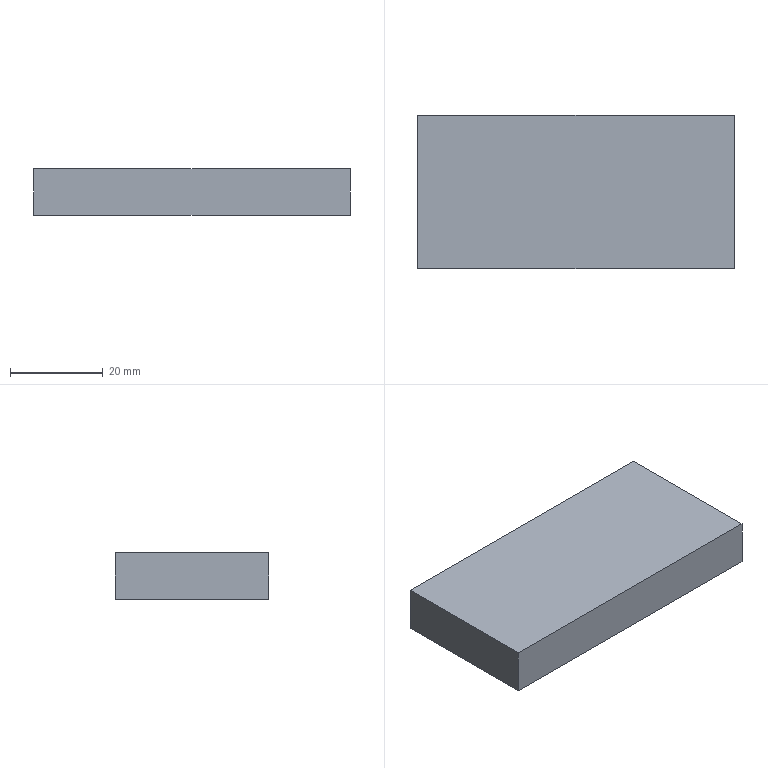Part | STEP file | Display 1 | 1 solid | 6 faces | box 68 x 33 x 10 mm | volume 22440 mm3 | plane 6
STEP:
#1=CARTESIAN_POINT('',(0.,0.,0.));
#2=DIRECTION('',(0.,0.,1.));
#3=DIRECTION('',(1.,0.,0.));
#4=AXIS2_PLACEMENT_3D('',#1,#2,#3);
#5=CARTESIAN_POINT('',(34.,-16.5,10.));
#6=VERTEX_POINT('',#5);
#7=CARTESIAN_POINT('',(34.,16.5,10.));
#8=VERTEX_POINT('',#7);
#9=CARTESIAN_POINT('',(34.,-16.5,10.));
#10=DIRECTION('',(0.,1.,0.));
#11=VECTOR('',#10,1.);
#12=LINE('',#9,#11);
#13=CARTESIAN_POINT('',(-34.,-16.5,10.));
#14=DIRECTION('',(0.,0.,1.));
#15=DIRECTION('',(1.,0.,0.));
#16=AXIS2_PLACEMENT_3D('',#13,#14,#15);
#17=PLANE('',#16);
#18=CARTESIAN_POINT('',(68.,0.));
#19=DIRECTION('',(0.,1.));
#20=VECTOR('',#19,1.);
#21=LINE('',#18,#20);
#22=(GEOMETRIC_REPRESENTATION_CONTEXT(2)PARAMETRIC_REPRESENTATION_CONTEXT()REPRESENTATION_CONTEXT('',''));
#23=DEFINITIONAL_REPRESENTATION('',(#21),#22);
#24=PCURVE('',#17,#23);
#25=CARTESIAN_POINT('',(34.,16.5,10.));
#26=DIRECTION('',(-1.,0.,0.));
#27=DIRECTION('',(0.,-1.,0.));
#28=AXIS2_PLACEMENT_3D('',#25,#26,#27);
#29=PLANE('',#28);
#30=CARTESIAN_POINT('',(33.,0.));
#31=DIRECTION('',(-1.,0.));
#32=VECTOR('',#31,1.);
#33=LINE('',#30,#32);
#34=(GEOMETRIC_REPRESENTATION_CONTEXT(2)PARAMETRIC_REPRESENTATION_CONTEXT()REPRESENTATION_CONTEXT('',''));
#35=DEFINITIONAL_REPRESENTATION('',(#33),#34);
#36=PCURVE('',#29,#35);
#37=SURFACE_CURVE('',#12,(#24,#36),.PCURVE_S1.);
#38=EDGE_CURVE('',#6,#8,#37,.T.);
#39=ORIENTED_EDGE('',*,*,#38,.T.);
#40=CARTESIAN_POINT('',(-34.,16.5,10.));
#41=VERTEX_POINT('',#40);
#42=CARTESIAN_POINT('',(-34.,16.5,10.));
#43=DIRECTION('',(-1.,0.,0.));
#44=VECTOR('',#43,1.);
#45=LINE('',#42,#44);
#46=CARTESIAN_POINT('',(0.,33.));
#47=DIRECTION('',(-1.,0.));
#48=VECTOR('',#47,1.);
#49=LINE('',#46,#48);
#50=(GEOMETRIC_REPRESENTATION_CONTEXT(2)PARAMETRIC_REPRESENTATION_CONTEXT()REPRESENTATION_CONTEXT('',''));
#51=DEFINITIONAL_REPRESENTATION('',(#49),#50);
#52=PCURVE('',#17,#51);
#53=CARTESIAN_POINT('',(-34.,16.5,10.));
#54=DIRECTION('',(0.,-1.,0.));
#55=DIRECTION('',(1.,0.,0.));
#56=AXIS2_PLACEMENT_3D('',#53,#54,#55);
#57=PLANE('',#56);
#58=CARTESIAN_POINT('',(0.,0.));
#59=DIRECTION('',(-1.,0.));
#60=VECTOR('',#59,1.);
#61=LINE('',#58,#60);
#62=(GEOMETRIC_REPRESENTATION_CONTEXT(2)PARAMETRIC_REPRESENTATION_CONTEXT()REPRESENTATION_CONTEXT('',''));
#63=DEFINITIONAL_REPRESENTATION('',(#61),#62);
#64=PCURVE('',#57,#63);
#65=SURFACE_CURVE('',#45,(#52,#64),.PCURVE_S1.);
#66=EDGE_CURVE('',#8,#41,#65,.T.);
#67=ORIENTED_EDGE('',*,*,#66,.T.);
#68=CARTESIAN_POINT('',(-34.,-16.5,10.));
#69=VERTEX_POINT('',#68);
#70=CARTESIAN_POINT('',(-34.,-16.5,10.));
#71=DIRECTION('',(0.,-1.,0.));
#72=VECTOR('',#71,1.);
#73=LINE('',#70,#72);
#74=CARTESIAN_POINT('',(0.,0.));
#75=DIRECTION('',(0.,-1.));
#76=VECTOR('',#75,1.);
#77=LINE('',#74,#76);
#78=(GEOMETRIC_REPRESENTATION_CONTEXT(2)PARAMETRIC_REPRESENTATION_CONTEXT()REPRESENTATION_CONTEXT('',''));
#79=DEFINITIONAL_REPRESENTATION('',(#77),#78);
#80=PCURVE('',#17,#79);
#81=CARTESIAN_POINT('',(-34.,16.5,10.));
#82=DIRECTION('',(1.,0.,0.));
#83=DIRECTION('',(0.,1.,0.));
#84=AXIS2_PLACEMENT_3D('',#81,#82,#83);
#85=PLANE('',#84);
#86=CARTESIAN_POINT('',(-33.,0.));
#87=DIRECTION('',(-1.,0.));
#88=VECTOR('',#87,1.);
#89=LINE('',#86,#88);
#90=(GEOMETRIC_REPRESENTATION_CONTEXT(2)PARAMETRIC_REPRESENTATION_CONTEXT()REPRESENTATION_CONTEXT('',''));
#91=DEFINITIONAL_REPRESENTATION('',(#89),#90);
#92=PCURVE('',#85,#91);
#93=SURFACE_CURVE('',#73,(#80,#92),.PCURVE_S1.);
#94=EDGE_CURVE('',#41,#69,#93,.T.);
#95=ORIENTED_EDGE('',*,*,#94,.T.);
#96=CARTESIAN_POINT('',(-34.,-16.5,10.));
#97=DIRECTION('',(1.,0.,0.));
#98=VECTOR('',#97,1.);
#99=LINE('',#96,#98);
#100=CARTESIAN_POINT('',(0.,0.));
#101=DIRECTION('',(1.,0.));
#102=VECTOR('',#101,1.);
#103=LINE('',#100,#102);
#104=(GEOMETRIC_REPRESENTATION_CONTEXT(2)PARAMETRIC_REPRESENTATION_CONTEXT()REPRESENTATION_CONTEXT('',''));
#105=DEFINITIONAL_REPRESENTATION('',(#103),#104);
#106=PCURVE('',#17,#105);
#107=CARTESIAN_POINT('',(-34.,-16.5,10.));
#108=DIRECTION('',(0.,1.,0.));
#109=DIRECTION('',(-1.,0.,0.));
#110=AXIS2_PLACEMENT_3D('',#107,#108,#109);
#111=PLANE('',#110);
#112=CARTESIAN_POINT('',(0.,0.));
#113=DIRECTION('',(-1.,0.));
#114=VECTOR('',#113,1.);
#115=LINE('',#112,#114);
#116=(GEOMETRIC_REPRESENTATION_CONTEXT(2)PARAMETRIC_REPRESENTATION_CONTEXT()REPRESENTATION_CONTEXT('',''));
#117=DEFINITIONAL_REPRESENTATION('',(#115),#116);
#118=PCURVE('',#111,#117);
#119=SURFACE_CURVE('',#99,(#106,#118),.PCURVE_S1.);
#120=EDGE_CURVE('',#69,#6,#119,.T.);
#121=ORIENTED_EDGE('',*,*,#120,.T.);
#122=EDGE_LOOP('',(#39,#67,#95,#121));
#123=FACE_BOUND('',#122,.T.);
#124=ADVANCED_FACE('',(#123),#17,.T.);
#125=CARTESIAN_POINT('',(-34.,16.5,0.));
#126=VERTEX_POINT('',#125);
#127=CARTESIAN_POINT('',(-34.,16.5,10.));
#128=DIRECTION('',(0.,0.,-1.));
#129=VECTOR('',#128,1.);
#130=LINE('',#127,#129);
#131=CARTESIAN_POINT('',(0.,0.));
#132=DIRECTION('',(0.,-1.));
#133=VECTOR('',#132,1.);
#134=LINE('',#131,#133);
#135=(GEOMETRIC_REPRESENTATION_CONTEXT(2)PARAMETRIC_REPRESENTATION_CONTEXT()REPRESENTATION_CONTEXT('',''));
#136=DEFINITIONAL_REPRESENTATION('',(#134),#135);
#137=PCURVE('',#57,#136);
#138=CARTESIAN_POINT('',(0.,0.));
#139=DIRECTION('',(0.,-1.));
#140=VECTOR('',#139,1.);
#141=LINE('',#138,#140);
#142=(GEOMETRIC_REPRESENTATION_CONTEXT(2)PARAMETRIC_REPRESENTATION_CONTEXT()REPRESENTATION_CONTEXT('',''));
#143=DEFINITIONAL_REPRESENTATION('',(#141),#142);
#144=PCURVE('',#85,#143);
#145=SURFACE_CURVE('',#130,(#137,#144),.PCURVE_S1.);
#146=EDGE_CURVE('',#41,#126,#145,.T.);
#147=ORIENTED_EDGE('',*,*,#146,.F.);
#148=ORIENTED_EDGE('',*,*,#66,.F.);
#149=CARTESIAN_POINT('',(34.,16.5,0.));
#150=VERTEX_POINT('',#149);
#151=CARTESIAN_POINT('',(34.,16.5,10.));
#152=DIRECTION('',(0.,0.,1.));
#153=VECTOR('',#152,1.);
#154=LINE('',#151,#153);
#155=CARTESIAN_POINT('',(68.,0.));
#156=DIRECTION('',(0.,1.));
#157=VECTOR('',#156,1.);
#158=LINE('',#155,#157);
#159=(GEOMETRIC_REPRESENTATION_CONTEXT(2)PARAMETRIC_REPRESENTATION_CONTEXT()REPRESENTATION_CONTEXT('',''));
#160=DEFINITIONAL_REPRESENTATION('',(#158),#159);
#161=PCURVE('',#57,#160);
#162=CARTESIAN_POINT('',(0.,0.));
#163=DIRECTION('',(0.,1.));
#164=VECTOR('',#163,1.);
#165=LINE('',#162,#164);
#166=(GEOMETRIC_REPRESENTATION_CONTEXT(2)PARAMETRIC_REPRESENTATION_CONTEXT()REPRESENTATION_CONTEXT('',''));
#167=DEFINITIONAL_REPRESENTATION('',(#165),#166);
#168=PCURVE('',#29,#167);
#169=SURFACE_CURVE('',#154,(#161,#168),.PCURVE_S1.);
#170=EDGE_CURVE('',#150,#8,#169,.T.);
#171=ORIENTED_EDGE('',*,*,#170,.F.);
#172=CARTESIAN_POINT('',(-34.,16.5,0.));
#173=DIRECTION('',(1.,0.,0.));
#174=VECTOR('',#173,1.);
#175=LINE('',#172,#174);
#176=CARTESIAN_POINT('',(0.,-10.));
#177=DIRECTION('',(1.,0.));
#178=VECTOR('',#177,1.);
#179=LINE('',#176,#178);
#180=(GEOMETRIC_REPRESENTATION_CONTEXT(2)PARAMETRIC_REPRESENTATION_CONTEXT()REPRESENTATION_CONTEXT('',''));
#181=DEFINITIONAL_REPRESENTATION('',(#179),#180);
#182=PCURVE('',#57,#181);
#183=CARTESIAN_POINT('',(-34.,-16.5,0.));
#184=DIRECTION('',(0.,0.,1.));
#185=DIRECTION('',(1.,0.,0.));
#186=AXIS2_PLACEMENT_3D('',#183,#184,#185);
#187=PLANE('',#186);
#188=CARTESIAN_POINT('',(0.,33.));
#189=DIRECTION('',(1.,0.));
#190=VECTOR('',#189,1.);
#191=LINE('',#188,#190);
#192=(GEOMETRIC_REPRESENTATION_CONTEXT(2)PARAMETRIC_REPRESENTATION_CONTEXT()REPRESENTATION_CONTEXT('',''));
#193=DEFINITIONAL_REPRESENTATION('',(#191),#192);
#194=PCURVE('',#187,#193);
#195=SURFACE_CURVE('',#175,(#182,#194),.PCURVE_S1.);
#196=EDGE_CURVE('',#126,#150,#195,.T.);
#197=ORIENTED_EDGE('',*,*,#196,.F.);
#198=EDGE_LOOP('',(#147,#148,#171,#197));
#199=FACE_BOUND('',#198,.T.);
#200=ADVANCED_FACE('',(#199),#57,.F.);
#201=ORIENTED_EDGE('',*,*,#170,.T.);
#202=ORIENTED_EDGE('',*,*,#38,.F.);
#203=CARTESIAN_POINT('',(34.,-16.5,0.));
#204=VERTEX_POINT('',#203);
#205=CARTESIAN_POINT('',(34.,-16.5,10.));
#206=DIRECTION('',(0.,0.,1.));
#207=VECTOR('',#206,1.);
#208=LINE('',#205,#207);
#209=CARTESIAN_POINT('',(33.,0.));
#210=DIRECTION('',(0.,1.));
#211=VECTOR('',#210,1.);
#212=LINE('',#209,#211);
#213=(GEOMETRIC_REPRESENTATION_CONTEXT(2)PARAMETRIC_REPRESENTATION_CONTEXT()REPRESENTATION_CONTEXT('',''));
#214=DEFINITIONAL_REPRESENTATION('',(#212),#213);
#215=PCURVE('',#29,#214);
#216=CARTESIAN_POINT('',(-68.,0.));
#217=DIRECTION('',(0.,1.));
#218=VECTOR('',#217,1.);
#219=LINE('',#216,#218);
#220=(GEOMETRIC_REPRESENTATION_CONTEXT(2)PARAMETRIC_REPRESENTATION_CONTEXT()REPRESENTATION_CONTEXT('',''));
#221=DEFINITIONAL_REPRESENTATION('',(#219),#220);
#222=PCURVE('',#111,#221);
#223=SURFACE_CURVE('',#208,(#215,#222),.PCURVE_S1.);
#224=EDGE_CURVE('',#204,#6,#223,.T.);
#225=ORIENTED_EDGE('',*,*,#224,.F.);
#226=CARTESIAN_POINT('',(34.,16.5,0.));
#227=DIRECTION('',(0.,-1.,0.));
#228=VECTOR('',#227,1.);
#229=LINE('',#226,#228);
#230=CARTESIAN_POINT('',(0.,-10.));
#231=DIRECTION('',(1.,0.));
#232=VECTOR('',#231,1.);
#233=LINE('',#230,#232);
#234=(GEOMETRIC_REPRESENTATION_CONTEXT(2)PARAMETRIC_REPRESENTATION_CONTEXT()REPRESENTATION_CONTEXT('',''));
#235=DEFINITIONAL_REPRESENTATION('',(#233),#234);
#236=PCURVE('',#29,#235);
#237=CARTESIAN_POINT('',(68.,33.));
#238=DIRECTION('',(0.,-1.));
#239=VECTOR('',#238,1.);
#240=LINE('',#237,#239);
#241=(GEOMETRIC_REPRESENTATION_CONTEXT(2)PARAMETRIC_REPRESENTATION_CONTEXT()REPRESENTATION_CONTEXT('',''));
#242=DEFINITIONAL_REPRESENTATION('',(#240),#241);
#243=PCURVE('',#187,#242);
#244=SURFACE_CURVE('',#229,(#236,#243),.PCURVE_S1.);
#245=EDGE_CURVE('',#150,#204,#244,.T.);
#246=ORIENTED_EDGE('',*,*,#245,.F.);
#247=EDGE_LOOP('',(#201,#202,#225,#246));
#248=FACE_BOUND('',#247,.T.);
#249=ADVANCED_FACE('',(#248),#29,.F.);
#250=ORIENTED_EDGE('',*,*,#224,.T.);
#251=ORIENTED_EDGE('',*,*,#120,.F.);
#252=CARTESIAN_POINT('',(-34.,-16.5,0.));
#253=VERTEX_POINT('',#252);
#254=CARTESIAN_POINT('',(-34.,-16.5,10.));
#255=DIRECTION('',(0.,0.,1.));
#256=VECTOR('',#255,1.);
#257=LINE('',#254,#256);
#258=CARTESIAN_POINT('',(0.,0.));
#259=DIRECTION('',(0.,1.));
#260=VECTOR('',#259,1.);
#261=LINE('',#258,#260);
#262=(GEOMETRIC_REPRESENTATION_CONTEXT(2)PARAMETRIC_REPRESENTATION_CONTEXT()REPRESENTATION_CONTEXT('',''));
#263=DEFINITIONAL_REPRESENTATION('',(#261),#262);
#264=PCURVE('',#111,#263);
#265=CARTESIAN_POINT('',(-33.,0.));
#266=DIRECTION('',(0.,1.));
#267=VECTOR('',#266,1.);
#268=LINE('',#265,#267);
#269=(GEOMETRIC_REPRESENTATION_CONTEXT(2)PARAMETRIC_REPRESENTATION_CONTEXT()REPRESENTATION_CONTEXT('',''));
#270=DEFINITIONAL_REPRESENTATION('',(#268),#269);
#271=PCURVE('',#85,#270);
#272=SURFACE_CURVE('',#257,(#264,#271),.PCURVE_S1.);
#273=EDGE_CURVE('',#253,#69,#272,.T.);
#274=ORIENTED_EDGE('',*,*,#273,.F.);
#275=CARTESIAN_POINT('',(-34.,-16.5,0.));
#276=DIRECTION('',(-1.,0.,0.));
#277=VECTOR('',#276,1.);
#278=LINE('',#275,#277);
#279=CARTESIAN_POINT('',(0.,-10.));
#280=DIRECTION('',(1.,0.));
#281=VECTOR('',#280,1.);
#282=LINE('',#279,#281);
#283=(GEOMETRIC_REPRESENTATION_CONTEXT(2)PARAMETRIC_REPRESENTATION_CONTEXT()REPRESENTATION_CONTEXT('',''));
#284=DEFINITIONAL_REPRESENTATION('',(#282),#283);
#285=PCURVE('',#111,#284);
#286=CARTESIAN_POINT('',(0.,0.));
#287=DIRECTION('',(-1.,0.));
#288=VECTOR('',#287,1.);
#289=LINE('',#286,#288);
#290=(GEOMETRIC_REPRESENTATION_CONTEXT(2)PARAMETRIC_REPRESENTATION_CONTEXT()REPRESENTATION_CONTEXT('',''));
#291=DEFINITIONAL_REPRESENTATION('',(#289),#290);
#292=PCURVE('',#187,#291);
#293=SURFACE_CURVE('',#278,(#285,#292),.PCURVE_S1.);
#294=EDGE_CURVE('',#204,#253,#293,.T.);
#295=ORIENTED_EDGE('',*,*,#294,.F.);
#296=EDGE_LOOP('',(#250,#251,#274,#295));
#297=FACE_BOUND('',#296,.T.);
#298=ADVANCED_FACE('',(#297),#111,.F.);
#299=ORIENTED_EDGE('',*,*,#273,.T.);
#300=ORIENTED_EDGE('',*,*,#94,.F.);
#301=ORIENTED_EDGE('',*,*,#146,.T.);
#302=CARTESIAN_POINT('',(-34.,16.5,0.));
#303=DIRECTION('',(0.,1.,0.));
#304=VECTOR('',#303,1.);
#305=LINE('',#302,#304);
#306=CARTESIAN_POINT('',(0.,-10.));
#307=DIRECTION('',(1.,0.));
#308=VECTOR('',#307,1.);
#309=LINE('',#306,#308);
#310=(GEOMETRIC_REPRESENTATION_CONTEXT(2)PARAMETRIC_REPRESENTATION_CONTEXT()REPRESENTATION_CONTEXT('',''));
#311=DEFINITIONAL_REPRESENTATION('',(#309),#310);
#312=PCURVE('',#85,#311);
#313=CARTESIAN_POINT('',(0.,33.));
#314=DIRECTION('',(0.,1.));
#315=VECTOR('',#314,1.);
#316=LINE('',#313,#315);
#317=(GEOMETRIC_REPRESENTATION_CONTEXT(2)PARAMETRIC_REPRESENTATION_CONTEXT()REPRESENTATION_CONTEXT('',''));
#318=DEFINITIONAL_REPRESENTATION('',(#316),#317);
#319=PCURVE('',#187,#318);
#320=SURFACE_CURVE('',#305,(#312,#319),.PCURVE_S1.);
#321=EDGE_CURVE('',#253,#126,#320,.T.);
#322=ORIENTED_EDGE('',*,*,#321,.F.);
#323=EDGE_LOOP('',(#299,#300,#301,#322));
#324=FACE_BOUND('',#323,.T.);
#325=ADVANCED_FACE('',(#324),#85,.F.);
#326=ORIENTED_EDGE('',*,*,#196,.T.);
#327=ORIENTED_EDGE('',*,*,#245,.T.);
#328=ORIENTED_EDGE('',*,*,#294,.T.);
#329=ORIENTED_EDGE('',*,*,#321,.T.);
#330=EDGE_LOOP('',(#326,#327,#328,#329));
#331=FACE_BOUND('',#330,.T.);
#332=ADVANCED_FACE('',(#331),#187,.F.);
#333=CLOSED_SHELL('',(#124,#200,#249,#298,#325,#332));
#334=MANIFOLD_SOLID_BREP('',#333);
#335=(LENGTH_UNIT()NAMED_UNIT(*)SI_UNIT(.MILLI.,.METRE.));
#336=UNCERTAINTY_MEASURE_WITH_UNIT(LENGTH_MEASURE(0.0000001),#335,'','');
#337=(NAMED_UNIT(*)PLANE_ANGLE_UNIT()SI_UNIT($,.RADIAN.));
#338=(NAMED_UNIT(*)SI_UNIT($,.STERADIAN.)SOLID_ANGLE_UNIT());
#339=(GEOMETRIC_REPRESENTATION_CONTEXT(3)GLOBAL_UNCERTAINTY_ASSIGNED_CONTEXT((#336))GLOBAL_UNIT_ASSIGNED_CONTEXT((#335,#337,#338))REPRESENTATION_CONTEXT('',''));
#340=ADVANCED_BREP_SHAPE_REPRESENTATION('',(#4,#334),#339);